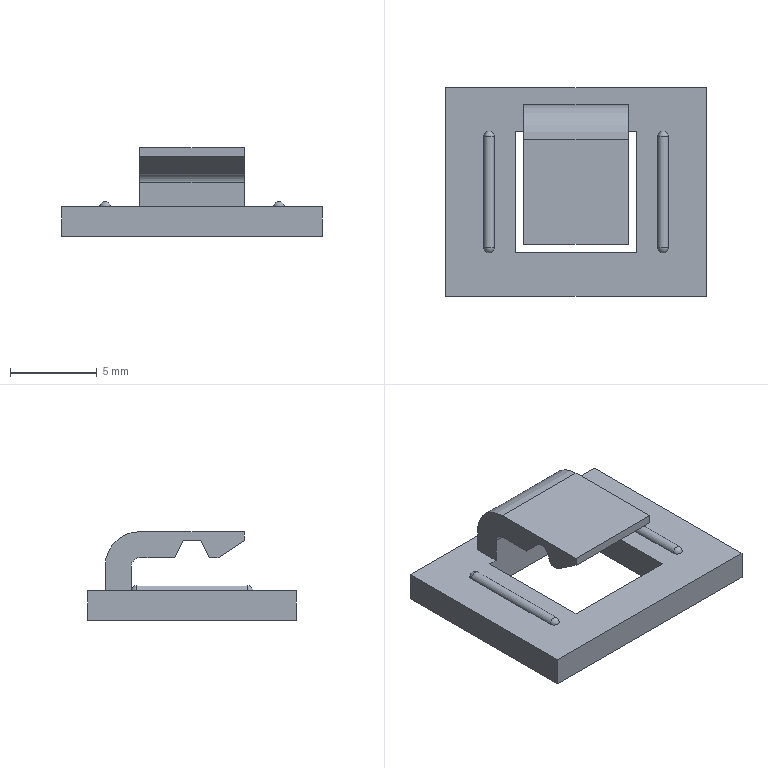Part | STEP file | Mount electronic clip, black, 20141015 | 1 solid | 29 faces | box 15 x 12 x 5.1 mm | volume 295.394 mm3 | plane 21 | cylinder 4 | sphere 4 | commonest cylinder face diameters 0.6 x2 1 x1 4 x1